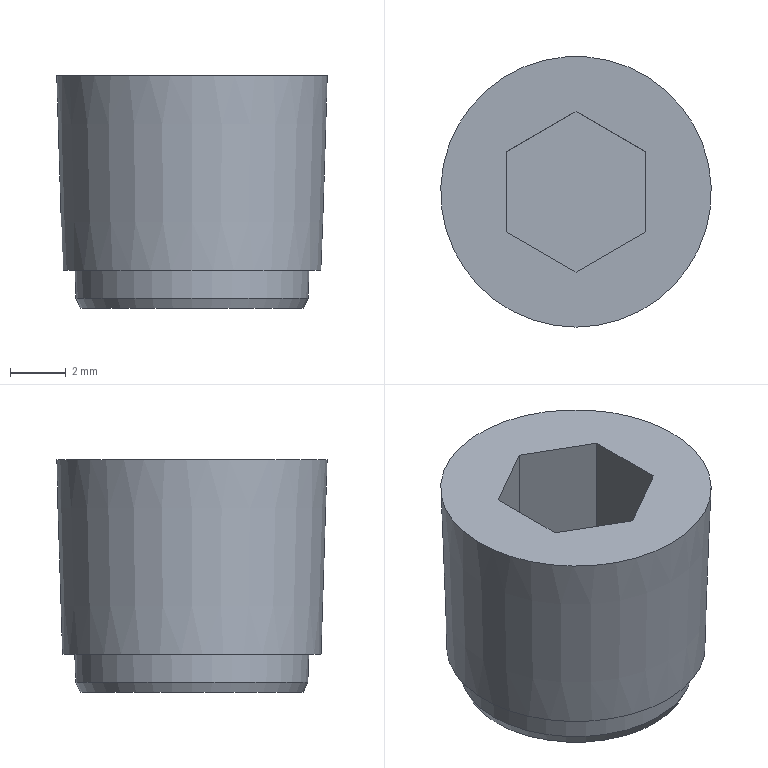Part | STEP file | EM31800001 | 1 solid | 13 faces | box 9.728 x 9.728 x 8.365 mm | volume 484.697 mm3 | plane 10 | cone 3
STEP:
#1=CARTESIAN_POINT('',(0.,0.,0.));
#2=DIRECTION('',(0.,0.,1.));
#3=DIRECTION('',(1.,0.,0.));
#4=AXIS2_PLACEMENT_3D('',#1,#2,#3);
#5=CARTESIAN_POINT('',(0.,-4.864,0.));
#6=VERTEX_POINT('',#5);
#7=CARTESIAN_POINT('',(0.,0.,0.));
#8=DIRECTION('',(0.,0.,-1.));
#9=DIRECTION('',(0.,-1.,0.));
#10=AXIS2_PLACEMENT_3D('',#7,#8,#9);
#11=CIRCLE('',#10,4.864);
#12=CARTESIAN_POINT('',(0.,0.,0.));
#13=DIRECTION('',(0.,0.,-1.));
#14=DIRECTION('',(0.,-1.,0.));
#15=AXIS2_PLACEMENT_3D('',#12,#13,#14);
#16=PLANE('',#15);
#17=CARTESIAN_POINT('',(0.,0.));
#18=DIRECTION('',(1.,0.));
#19=AXIS2_PLACEMENT_2D('',#17,#18);
#20=CIRCLE('',#19,4.864);
#21=(GEOMETRIC_REPRESENTATION_CONTEXT(2)PARAMETRIC_REPRESENTATION_CONTEXT()REPRESENTATION_CONTEXT('',''));
#22=DEFINITIONAL_REPRESENTATION('',(#20),#21);
#23=PCURVE('',#16,#22);
#24=CARTESIAN_POINT('',(0.,0.,-6.997));
#25=DIRECTION('',(0.,0.,1.));
#26=DIRECTION('',(0.,1.,0.));
#27=AXIS2_PLACEMENT_3D('',#24,#25,#26);
#28=CONICAL_SURFACE('',#27,4.644,0.03142);
#29=CARTESIAN_POINT('',(9.425,6.997));
#30=DIRECTION('',(-1.,0.));
#31=VECTOR('',#30,1.);
#32=LINE('',#29,#31);
#33=(GEOMETRIC_REPRESENTATION_CONTEXT(2)PARAMETRIC_REPRESENTATION_CONTEXT()REPRESENTATION_CONTEXT('',''));
#34=DEFINITIONAL_REPRESENTATION('',(#32),#33);
#35=PCURVE('',#28,#34);
#36=SURFACE_CURVE('',#11,(#23,#35),.PCURVE_S1.);
#37=EDGE_CURVE('',#6,#6,#36,.T.);
#38=ORIENTED_EDGE('',*,*,#37,.F.);
#39=EDGE_LOOP('',(#38));
#40=FACE_BOUND('',#39,.T.);
#41=CARTESIAN_POINT('',(0.,2.887,0.));
#42=VERTEX_POINT('',#41);
#43=CARTESIAN_POINT('',(-2.5,1.443,0.));
#44=VERTEX_POINT('',#43);
#45=CARTESIAN_POINT('',(-1.25,2.165,0.));
#46=DIRECTION('',(-0.866,-0.5,0.));
#47=VECTOR('',#46,1.);
#48=LINE('',#45,#47);
#49=CARTESIAN_POINT('',(-2.165,1.25));
#50=DIRECTION('',(0.5,0.866));
#51=VECTOR('',#50,1.);
#52=LINE('',#49,#51);
#53=(GEOMETRIC_REPRESENTATION_CONTEXT(2)PARAMETRIC_REPRESENTATION_CONTEXT()REPRESENTATION_CONTEXT('',''));
#54=DEFINITIONAL_REPRESENTATION('',(#52),#53);
#55=PCURVE('',#16,#54);
#56=CARTESIAN_POINT('',(-2.5,1.443,-5.));
#57=DIRECTION('',(0.5,-0.866,0.));
#58=DIRECTION('',(-0.866,-0.5,0.));
#59=AXIS2_PLACEMENT_3D('',#56,#57,#58);
#60=PLANE('',#59);
#61=CARTESIAN_POINT('',(-1.443,-5.));
#62=DIRECTION('',(1.,0.));
#63=VECTOR('',#62,1.);
#64=LINE('',#61,#63);
#65=(GEOMETRIC_REPRESENTATION_CONTEXT(2)PARAMETRIC_REPRESENTATION_CONTEXT()REPRESENTATION_CONTEXT('',''));
#66=DEFINITIONAL_REPRESENTATION('',(#64),#65);
#67=PCURVE('',#60,#66);
#68=SURFACE_CURVE('',#48,(#55,#67),.PCURVE_S1.);
#69=EDGE_CURVE('',#42,#44,#68,.T.);
#70=ORIENTED_EDGE('',*,*,#69,.F.);
#71=CARTESIAN_POINT('',(2.5,1.443,0.));
#72=VERTEX_POINT('',#71);
#73=CARTESIAN_POINT('',(1.25,2.165,0.));
#74=DIRECTION('',(-0.866,0.5,0.));
#75=VECTOR('',#74,1.);
#76=LINE('',#73,#75);
#77=CARTESIAN_POINT('',(-2.165,-1.25));
#78=DIRECTION('',(-0.5,0.866));
#79=VECTOR('',#78,1.);
#80=LINE('',#77,#79);
#81=(GEOMETRIC_REPRESENTATION_CONTEXT(2)PARAMETRIC_REPRESENTATION_CONTEXT()REPRESENTATION_CONTEXT('',''));
#82=DEFINITIONAL_REPRESENTATION('',(#80),#81);
#83=PCURVE('',#16,#82);
#84=CARTESIAN_POINT('',(0.,2.887,-5.));
#85=DIRECTION('',(-0.5,-0.866,0.));
#86=DIRECTION('',(-0.866,0.5,0.));
#87=AXIS2_PLACEMENT_3D('',#84,#85,#86);
#88=PLANE('',#87);
#89=CARTESIAN_POINT('',(-1.443,-5.));
#90=DIRECTION('',(1.,0.));
#91=VECTOR('',#90,1.);
#92=LINE('',#89,#91);
#93=(GEOMETRIC_REPRESENTATION_CONTEXT(2)PARAMETRIC_REPRESENTATION_CONTEXT()REPRESENTATION_CONTEXT('',''));
#94=DEFINITIONAL_REPRESENTATION('',(#92),#93);
#95=PCURVE('',#88,#94);
#96=SURFACE_CURVE('',#76,(#83,#95),.PCURVE_S1.);
#97=EDGE_CURVE('',#72,#42,#96,.T.);
#98=ORIENTED_EDGE('',*,*,#97,.F.);
#99=CARTESIAN_POINT('',(2.5,-1.443,0.));
#100=VERTEX_POINT('',#99);
#101=CARTESIAN_POINT('',(2.5,0.,0.));
#102=DIRECTION('',(0.,1.,0.));
#103=VECTOR('',#102,1.);
#104=LINE('',#101,#103);
#105=CARTESIAN_POINT('',(0.,-2.5));
#106=DIRECTION('',(-1.,0.));
#107=VECTOR('',#106,1.);
#108=LINE('',#105,#107);
#109=(GEOMETRIC_REPRESENTATION_CONTEXT(2)PARAMETRIC_REPRESENTATION_CONTEXT()REPRESENTATION_CONTEXT('',''));
#110=DEFINITIONAL_REPRESENTATION('',(#108),#109);
#111=PCURVE('',#16,#110);
#112=CARTESIAN_POINT('',(2.5,1.443,-5.));
#113=DIRECTION('',(-1.,0.,0.));
#114=DIRECTION('',(0.,1.,0.));
#115=AXIS2_PLACEMENT_3D('',#112,#113,#114);
#116=PLANE('',#115);
#117=CARTESIAN_POINT('',(-1.443,-5.));
#118=DIRECTION('',(1.,0.));
#119=VECTOR('',#118,1.);
#120=LINE('',#117,#119);
#121=(GEOMETRIC_REPRESENTATION_CONTEXT(2)PARAMETRIC_REPRESENTATION_CONTEXT()REPRESENTATION_CONTEXT('',''));
#122=DEFINITIONAL_REPRESENTATION('',(#120),#121);
#123=PCURVE('',#116,#122);
#124=SURFACE_CURVE('',#104,(#111,#123),.PCURVE_S1.);
#125=EDGE_CURVE('',#100,#72,#124,.T.);
#126=ORIENTED_EDGE('',*,*,#125,.F.);
#127=CARTESIAN_POINT('',(0.,-2.887,0.));
#128=VERTEX_POINT('',#127);
#129=CARTESIAN_POINT('',(1.25,-2.165,0.));
#130=DIRECTION('',(0.866,0.5,0.));
#131=VECTOR('',#130,1.);
#132=LINE('',#129,#131);
#133=CARTESIAN_POINT('',(2.165,-1.25));
#134=DIRECTION('',(-0.5,-0.866));
#135=VECTOR('',#134,1.);
#136=LINE('',#133,#135);
#137=(GEOMETRIC_REPRESENTATION_CONTEXT(2)PARAMETRIC_REPRESENTATION_CONTEXT()REPRESENTATION_CONTEXT('',''));
#138=DEFINITIONAL_REPRESENTATION('',(#136),#137);
#139=PCURVE('',#16,#138);
#140=CARTESIAN_POINT('',(2.5,-1.443,-5.));
#141=DIRECTION('',(-0.5,0.866,0.));
#142=DIRECTION('',(0.866,0.5,0.));
#143=AXIS2_PLACEMENT_3D('',#140,#141,#142);
#144=PLANE('',#143);
#145=CARTESIAN_POINT('',(-1.443,-5.));
#146=DIRECTION('',(1.,0.));
#147=VECTOR('',#146,1.);
#148=LINE('',#145,#147);
#149=(GEOMETRIC_REPRESENTATION_CONTEXT(2)PARAMETRIC_REPRESENTATION_CONTEXT()REPRESENTATION_CONTEXT('',''));
#150=DEFINITIONAL_REPRESENTATION('',(#148),#149);
#151=PCURVE('',#144,#150);
#152=SURFACE_CURVE('',#132,(#139,#151),.PCURVE_S1.);
#153=EDGE_CURVE('',#128,#100,#152,.T.);
#154=ORIENTED_EDGE('',*,*,#153,.F.);
#155=CARTESIAN_POINT('',(-2.5,-1.443,0.));
#156=VERTEX_POINT('',#155);
#157=CARTESIAN_POINT('',(-1.25,-2.165,0.));
#158=DIRECTION('',(0.866,-0.5,0.));
#159=VECTOR('',#158,1.);
#160=LINE('',#157,#159);
#161=CARTESIAN_POINT('',(2.165,1.25));
#162=DIRECTION('',(0.5,-0.866));
#163=VECTOR('',#162,1.);
#164=LINE('',#161,#163);
#165=(GEOMETRIC_REPRESENTATION_CONTEXT(2)PARAMETRIC_REPRESENTATION_CONTEXT()REPRESENTATION_CONTEXT('',''));
#166=DEFINITIONAL_REPRESENTATION('',(#164),#165);
#167=PCURVE('',#16,#166);
#168=CARTESIAN_POINT('',(0.,-2.887,-5.));
#169=DIRECTION('',(0.5,0.866,0.));
#170=DIRECTION('',(0.866,-0.5,0.));
#171=AXIS2_PLACEMENT_3D('',#168,#169,#170);
#172=PLANE('',#171);
#173=CARTESIAN_POINT('',(-1.443,-5.));
#174=DIRECTION('',(1.,0.));
#175=VECTOR('',#174,1.);
#176=LINE('',#173,#175);
#177=(GEOMETRIC_REPRESENTATION_CONTEXT(2)PARAMETRIC_REPRESENTATION_CONTEXT()REPRESENTATION_CONTEXT('',''));
#178=DEFINITIONAL_REPRESENTATION('',(#176),#177);
#179=PCURVE('',#172,#178);
#180=SURFACE_CURVE('',#160,(#167,#179),.PCURVE_S1.);
#181=EDGE_CURVE('',#156,#128,#180,.T.);
#182=ORIENTED_EDGE('',*,*,#181,.F.);
#183=CARTESIAN_POINT('',(-2.5,0.,0.));
#184=DIRECTION('',(0.,-1.,0.));
#185=VECTOR('',#184,1.);
#186=LINE('',#183,#185);
#187=CARTESIAN_POINT('',(0.,2.5));
#188=DIRECTION('',(1.,0.));
#189=VECTOR('',#188,1.);
#190=LINE('',#187,#189);
#191=(GEOMETRIC_REPRESENTATION_CONTEXT(2)PARAMETRIC_REPRESENTATION_CONTEXT()REPRESENTATION_CONTEXT('',''));
#192=DEFINITIONAL_REPRESENTATION('',(#190),#191);
#193=PCURVE('',#16,#192);
#194=CARTESIAN_POINT('',(-2.5,-1.443,-5.));
#195=DIRECTION('',(1.,0.,0.));
#196=DIRECTION('',(0.,-1.,0.));
#197=AXIS2_PLACEMENT_3D('',#194,#195,#196);
#198=PLANE('',#197);
#199=CARTESIAN_POINT('',(-1.443,-5.));
#200=DIRECTION('',(1.,0.));
#201=VECTOR('',#200,1.);
#202=LINE('',#199,#201);
#203=(GEOMETRIC_REPRESENTATION_CONTEXT(2)PARAMETRIC_REPRESENTATION_CONTEXT()REPRESENTATION_CONTEXT('',''));
#204=DEFINITIONAL_REPRESENTATION('',(#202),#203);
#205=PCURVE('',#198,#204);
#206=SURFACE_CURVE('',#186,(#193,#205),.PCURVE_S1.);
#207=EDGE_CURVE('',#44,#156,#206,.T.);
#208=ORIENTED_EDGE('',*,*,#207,.F.);
#209=EDGE_LOOP('',(#70,#98,#126,#154,#182,#208));
#210=FACE_BOUND('',#209,.T.);
#211=ADVANCED_FACE('',(#40,#210),#16,.F.);
#212=CARTESIAN_POINT('',(0.,-4.644,-6.997));
#213=VERTEX_POINT('',#212);
#214=CARTESIAN_POINT('',(0.,0.,-6.997));
#215=DIRECTION('',(0.,0.,-1.));
#216=DIRECTION('',(0.,-1.,0.));
#217=AXIS2_PLACEMENT_3D('',#214,#215,#216);
#218=CIRCLE('',#217,4.644);
#219=CARTESIAN_POINT('',(0.,0.,-6.997));
#220=DIRECTION('',(0.,0.,-1.));
#221=DIRECTION('',(0.,-1.,0.));
#222=AXIS2_PLACEMENT_3D('',#219,#220,#221);
#223=PLANE('',#222);
#224=CARTESIAN_POINT('',(0.,0.));
#225=DIRECTION('',(1.,0.));
#226=AXIS2_PLACEMENT_2D('',#224,#225);
#227=CIRCLE('',#226,4.644);
#228=(GEOMETRIC_REPRESENTATION_CONTEXT(2)PARAMETRIC_REPRESENTATION_CONTEXT()REPRESENTATION_CONTEXT('',''));
#229=DEFINITIONAL_REPRESENTATION('',(#227),#228);
#230=PCURVE('',#223,#229);
#231=CARTESIAN_POINT('',(9.425,0.));
#232=DIRECTION('',(-1.,0.));
#233=VECTOR('',#232,1.);
#234=LINE('',#231,#233);
#235=(GEOMETRIC_REPRESENTATION_CONTEXT(2)PARAMETRIC_REPRESENTATION_CONTEXT()REPRESENTATION_CONTEXT('',''));
#236=DEFINITIONAL_REPRESENTATION('',(#234),#235);
#237=PCURVE('',#28,#236);
#238=SURFACE_CURVE('',#218,(#230,#237),.PCURVE_S1.);
#239=EDGE_CURVE('',#213,#213,#238,.T.);
#240=ORIENTED_EDGE('',*,*,#239,.T.);
#241=EDGE_LOOP('',(#240));
#242=FACE_BOUND('',#241,.T.);
#243=CARTESIAN_POINT('',(0.,-4.204,-6.997));
#244=VERTEX_POINT('',#243);
#245=CARTESIAN_POINT('',(0.,0.,-6.997));
#246=DIRECTION('',(0.,0.,1.));
#247=DIRECTION('',(0.,-1.,0.));
#248=AXIS2_PLACEMENT_3D('',#245,#246,#247);
#249=CIRCLE('',#248,4.204);
#250=CARTESIAN_POINT('',(4.204,0.));
#251=CARTESIAN_POINT('',(4.204,-7.281));
#252=CARTESIAN_POINT('',(-2.102,-3.641));
#253=CARTESIAN_POINT('',(-8.407,0.));
#254=CARTESIAN_POINT('',(-2.102,3.641));
#255=CARTESIAN_POINT('',(4.204,7.281));
#256=CARTESIAN_POINT('',(4.204,0.));
#257=(BOUNDED_CURVE()B_SPLINE_CURVE(2,(#250,#251,#252,#253,#254,#255,#256),.UNSPECIFIED.,.T.,.F.)B_SPLINE_CURVE_WITH_KNOTS((1,2,2,2,2,1),(-2.094,0.,2.094,4.189,6.283,8.378),.UNSPECIFIED.)CURVE()GEOMETRIC_REPRESENTATION_ITEM()RATIONAL_B_SPLINE_CURVE((1.,0.5,1.,0.5,1.,0.5,1.))REPRESENTATION_ITEM(''));
#258=(GEOMETRIC_REPRESENTATION_CONTEXT(2)PARAMETRIC_REPRESENTATION_CONTEXT()REPRESENTATION_CONTEXT('',''));
#259=DEFINITIONAL_REPRESENTATION('',(#257),#258);
#260=PCURVE('',#223,#259);
#261=CARTESIAN_POINT('',(0.,0.,-7.997));
#262=DIRECTION('',(0.,0.,1.));
#263=DIRECTION('',(0.,1.,0.));
#264=AXIS2_PLACEMENT_3D('',#261,#262,#263);
#265=CONICAL_SURFACE('',#264,4.172,0.03142);
#266=CARTESIAN_POINT('',(3.142,1.001));
#267=DIRECTION('',(1.,0.));
#268=VECTOR('',#267,1.);
#269=LINE('',#266,#268);
#270=(GEOMETRIC_REPRESENTATION_CONTEXT(2)PARAMETRIC_REPRESENTATION_CONTEXT()REPRESENTATION_CONTEXT('',''));
#271=DEFINITIONAL_REPRESENTATION('',(#269),#270);
#272=PCURVE('',#265,#271);
#273=SURFACE_CURVE('',#249,(#260,#272),.PCURVE_S1.);
#274=EDGE_CURVE('',#244,#244,#273,.T.);
#275=ORIENTED_EDGE('',*,*,#274,.T.);
#276=EDGE_LOOP('',(#275));
#277=FACE_BOUND('',#276,.T.);
#278=ADVANCED_FACE('',(#242,#277),#223,.T.);
#279=ORIENTED_EDGE('',*,*,#37,.T.);
#280=CARTESIAN_POINT('',(0.,-4.644,-6.997));
#281=CARTESIAN_POINT('',(0.,-4.864,0.));
#282=B_SPLINE_CURVE_WITH_KNOTS('',1,(#280,#281),.UNSPECIFIED.,.F.,.F.,(2,2),(0.,7.),.PIECEWISE_BEZIER_KNOTS.);
#283=CARTESIAN_POINT('',(3.142,0.));
#284=DIRECTION('',(0.,1.));
#285=VECTOR('',#284,1.);
#286=LINE('',#283,#285);
#287=(GEOMETRIC_REPRESENTATION_CONTEXT(2)PARAMETRIC_REPRESENTATION_CONTEXT()REPRESENTATION_CONTEXT('',''));
#288=DEFINITIONAL_REPRESENTATION('',(#286),#287);
#289=PCURVE('',#28,#288);
#290=CARTESIAN_POINT('',(9.425,0.));
#291=DIRECTION('',(0.,1.));
#292=VECTOR('',#291,1.);
#293=LINE('',#290,#292);
#294=(GEOMETRIC_REPRESENTATION_CONTEXT(2)PARAMETRIC_REPRESENTATION_CONTEXT()REPRESENTATION_CONTEXT('',''));
#295=DEFINITIONAL_REPRESENTATION('',(#293),#294);
#296=PCURVE('',#28,#295);
#297=SEAM_CURVE('',#282,(#289,#296),.PCURVE_S1.);
#298=EDGE_CURVE('',#213,#6,#297,.T.);
#299=ORIENTED_EDGE('',*,*,#298,.F.);
#300=ORIENTED_EDGE('',*,*,#239,.F.);
#301=ORIENTED_EDGE('',*,*,#298,.T.);
#302=EDGE_LOOP('',(#279,#299,#300,#301));
#303=FACE_BOUND('',#302,.T.);
#304=ADVANCED_FACE('',(#303),#28,.T.);
#305=ORIENTED_EDGE('',*,*,#274,.F.);
#306=CARTESIAN_POINT('',(0.,-4.172,-7.997));
#307=VERTEX_POINT('',#306);
#308=CARTESIAN_POINT('',(0.,-4.172,-7.997));
#309=CARTESIAN_POINT('',(0.,-4.204,-6.997));
#310=B_SPLINE_CURVE_WITH_KNOTS('',1,(#308,#309),.UNSPECIFIED.,.F.,.F.,(2,2),(0.,1.001),.PIECEWISE_BEZIER_KNOTS.);
#311=CARTESIAN_POINT('',(3.142,0.));
#312=DIRECTION('',(0.,1.));
#313=VECTOR('',#312,1.);
#314=LINE('',#311,#313);
#315=(GEOMETRIC_REPRESENTATION_CONTEXT(2)PARAMETRIC_REPRESENTATION_CONTEXT()REPRESENTATION_CONTEXT('',''));
#316=DEFINITIONAL_REPRESENTATION('',(#314),#315);
#317=PCURVE('',#265,#316);
#318=CARTESIAN_POINT('',(9.425,0.));
#319=DIRECTION('',(0.,1.));
#320=VECTOR('',#319,1.);
#321=LINE('',#318,#320);
#322=(GEOMETRIC_REPRESENTATION_CONTEXT(2)PARAMETRIC_REPRESENTATION_CONTEXT()REPRESENTATION_CONTEXT('',''));
#323=DEFINITIONAL_REPRESENTATION('',(#321),#322);
#324=PCURVE('',#265,#323);
#325=SEAM_CURVE('',#310,(#317,#324),.PCURVE_S1.);
#326=EDGE_CURVE('',#307,#244,#325,.T.);
#327=ORIENTED_EDGE('',*,*,#326,.F.);
#328=CARTESIAN_POINT('',(0.,0.,-7.997));
#329=DIRECTION('',(0.,0.,-1.));
#330=DIRECTION('',(0.,-1.,0.));
#331=AXIS2_PLACEMENT_3D('',#328,#329,#330);
#332=CIRCLE('',#331,4.172);
#333=CARTESIAN_POINT('',(9.425,0.));
#334=DIRECTION('',(-1.,0.));
#335=VECTOR('',#334,1.);
#336=LINE('',#333,#335);
#337=(GEOMETRIC_REPRESENTATION_CONTEXT(2)PARAMETRIC_REPRESENTATION_CONTEXT()REPRESENTATION_CONTEXT('',''));
#338=DEFINITIONAL_REPRESENTATION('',(#336),#337);
#339=PCURVE('',#265,#338);
#340=CARTESIAN_POINT('',(0.,0.,-8.365));
#341=DIRECTION('',(0.,0.,1.));
#342=DIRECTION('',(0.,1.,0.));
#343=AXIS2_PLACEMENT_3D('',#340,#341,#342);
#344=CONICAL_SURFACE('',#343,4.,0.4379);
#345=CARTESIAN_POINT('',(9.425,0.3679));
#346=DIRECTION('',(-1.,0.));
#347=VECTOR('',#346,1.);
#348=LINE('',#345,#347);
#349=(GEOMETRIC_REPRESENTATION_CONTEXT(2)PARAMETRIC_REPRESENTATION_CONTEXT()REPRESENTATION_CONTEXT('',''));
#350=DEFINITIONAL_REPRESENTATION('',(#348),#349);
#351=PCURVE('',#344,#350);
#352=SURFACE_CURVE('',#332,(#339,#351),.PCURVE_S1.);
#353=EDGE_CURVE('',#307,#307,#352,.T.);
#354=ORIENTED_EDGE('',*,*,#353,.F.);
#355=ORIENTED_EDGE('',*,*,#326,.T.);
#356=EDGE_LOOP('',(#305,#327,#354,#355));
#357=FACE_BOUND('',#356,.T.);
#358=ADVANCED_FACE('',(#357),#265,.T.);
#359=ORIENTED_EDGE('',*,*,#353,.T.);
#360=CARTESIAN_POINT('',(0.,-4.,-8.365));
#361=VERTEX_POINT('',#360);
#362=CARTESIAN_POINT('',(0.,-4.,-8.365));
#363=CARTESIAN_POINT('',(0.,-4.172,-7.997));
#364=B_SPLINE_CURVE_WITH_KNOTS('',1,(#362,#363),.UNSPECIFIED.,.F.,.F.,(2,2),(0.,0.4063),.PIECEWISE_BEZIER_KNOTS.);
#365=CARTESIAN_POINT('',(3.142,0.));
#366=DIRECTION('',(0.,1.));
#367=VECTOR('',#366,1.);
#368=LINE('',#365,#367);
#369=(GEOMETRIC_REPRESENTATION_CONTEXT(2)PARAMETRIC_REPRESENTATION_CONTEXT()REPRESENTATION_CONTEXT('',''));
#370=DEFINITIONAL_REPRESENTATION('',(#368),#369);
#371=PCURVE('',#344,#370);
#372=CARTESIAN_POINT('',(9.425,0.));
#373=DIRECTION('',(0.,1.));
#374=VECTOR('',#373,1.);
#375=LINE('',#372,#374);
#376=(GEOMETRIC_REPRESENTATION_CONTEXT(2)PARAMETRIC_REPRESENTATION_CONTEXT()REPRESENTATION_CONTEXT('',''));
#377=DEFINITIONAL_REPRESENTATION('',(#375),#376);
#378=PCURVE('',#344,#377);
#379=SEAM_CURVE('',#364,(#371,#378),.PCURVE_S1.);
#380=EDGE_CURVE('',#361,#307,#379,.T.);
#381=ORIENTED_EDGE('',*,*,#380,.F.);
#382=CARTESIAN_POINT('',(0.,0.,-8.365));
#383=DIRECTION('',(0.,0.,-1.));
#384=DIRECTION('',(0.,-1.,0.));
#385=AXIS2_PLACEMENT_3D('',#382,#383,#384);
#386=CIRCLE('',#385,4.);
#387=CARTESIAN_POINT('',(9.425,0.));
#388=DIRECTION('',(-1.,0.));
#389=VECTOR('',#388,1.);
#390=LINE('',#387,#389);
#391=(GEOMETRIC_REPRESENTATION_CONTEXT(2)PARAMETRIC_REPRESENTATION_CONTEXT()REPRESENTATION_CONTEXT('',''));
#392=DEFINITIONAL_REPRESENTATION('',(#390),#391);
#393=PCURVE('',#344,#392);
#394=CARTESIAN_POINT('',(0.,0.,-8.365));
#395=DIRECTION('',(0.,0.,-1.));
#396=DIRECTION('',(0.,-1.,0.));
#397=AXIS2_PLACEMENT_3D('',#394,#395,#396);
#398=PLANE('',#397);
#399=CARTESIAN_POINT('',(0.,0.));
#400=DIRECTION('',(1.,0.));
#401=AXIS2_PLACEMENT_2D('',#399,#400);
#402=CIRCLE('',#401,4.);
#403=(GEOMETRIC_REPRESENTATION_CONTEXT(2)PARAMETRIC_REPRESENTATION_CONTEXT()REPRESENTATION_CONTEXT('',''));
#404=DEFINITIONAL_REPRESENTATION('',(#402),#403);
#405=PCURVE('',#398,#404);
#406=SURFACE_CURVE('',#386,(#393,#405),.PCURVE_S1.);
#407=EDGE_CURVE('',#361,#361,#406,.T.);
#408=ORIENTED_EDGE('',*,*,#407,.F.);
#409=ORIENTED_EDGE('',*,*,#380,.T.);
#410=EDGE_LOOP('',(#359,#381,#408,#409));
#411=FACE_BOUND('',#410,.T.);
#412=ADVANCED_FACE('',(#411),#344,.T.);
#413=ORIENTED_EDGE('',*,*,#407,.T.);
#414=EDGE_LOOP('',(#413));
#415=FACE_BOUND('',#414,.T.);
#416=ADVANCED_FACE('',(#415),#398,.T.);
#417=ORIENTED_EDGE('',*,*,#69,.T.);
#418=CARTESIAN_POINT('',(-2.5,1.443,-4.));
#419=VERTEX_POINT('',#418);
#420=CARTESIAN_POINT('',(-2.5,1.443,-5.));
#421=DIRECTION('',(0.,0.,1.));
#422=VECTOR('',#421,1.);
#423=LINE('',#420,#422);
#424=CARTESIAN_POINT('',(0.,0.));
#425=DIRECTION('',(0.,-1.));
#426=VECTOR('',#425,1.);
#427=LINE('',#424,#426);
#428=(GEOMETRIC_REPRESENTATION_CONTEXT(2)PARAMETRIC_REPRESENTATION_CONTEXT()REPRESENTATION_CONTEXT('',''));
#429=DEFINITIONAL_REPRESENTATION('',(#427),#428);
#430=PCURVE('',#60,#429);
#431=CARTESIAN_POINT('',(-2.887,0.));
#432=DIRECTION('',(0.,-1.));
#433=VECTOR('',#432,1.);
#434=LINE('',#431,#433);
#435=(GEOMETRIC_REPRESENTATION_CONTEXT(2)PARAMETRIC_REPRESENTATION_CONTEXT()REPRESENTATION_CONTEXT('',''));
#436=DEFINITIONAL_REPRESENTATION('',(#434),#435);
#437=PCURVE('',#198,#436);
#438=SURFACE_CURVE('',#423,(#430,#437),.PCURVE_S1.);
#439=EDGE_CURVE('',#419,#44,#438,.T.);
#440=ORIENTED_EDGE('',*,*,#439,.F.);
#441=CARTESIAN_POINT('',(0.,2.887,-4.));
#442=VERTEX_POINT('',#441);
#443=CARTESIAN_POINT('',(-1.25,2.165,-4.));
#444=DIRECTION('',(0.866,0.5,0.));
#445=VECTOR('',#444,1.);
#446=LINE('',#443,#445);
#447=CARTESIAN_POINT('',(-1.443,-1.));
#448=DIRECTION('',(-1.,0.));
#449=VECTOR('',#448,1.);
#450=LINE('',#447,#449);
#451=(GEOMETRIC_REPRESENTATION_CONTEXT(2)PARAMETRIC_REPRESENTATION_CONTEXT()REPRESENTATION_CONTEXT('',''));
#452=DEFINITIONAL_REPRESENTATION('',(#450),#451);
#453=PCURVE('',#60,#452);
#454=CARTESIAN_POINT('',(-1.25,2.165,-4.));
#455=DIRECTION('',(0.,0.,1.));
#456=DIRECTION('',(0.,1.,0.));
#457=AXIS2_PLACEMENT_3D('',#454,#455,#456);
#458=PLANE('',#457);
#459=CARTESIAN_POINT('',(0.,0.));
#460=DIRECTION('',(0.5,-0.866));
#461=VECTOR('',#460,1.);
#462=LINE('',#459,#461);
#463=(GEOMETRIC_REPRESENTATION_CONTEXT(2)PARAMETRIC_REPRESENTATION_CONTEXT()REPRESENTATION_CONTEXT('',''));
#464=DEFINITIONAL_REPRESENTATION('',(#462),#463);
#465=PCURVE('',#458,#464);
#466=SURFACE_CURVE('',#446,(#453,#465),.PCURVE_S1.);
#467=EDGE_CURVE('',#419,#442,#466,.T.);
#468=ORIENTED_EDGE('',*,*,#467,.T.);
#469=CARTESIAN_POINT('',(0.,2.887,-5.));
#470=DIRECTION('',(0.,0.,1.));
#471=VECTOR('',#470,1.);
#472=LINE('',#469,#471);
#473=CARTESIAN_POINT('',(-2.887,0.));
#474=DIRECTION('',(0.,-1.));
#475=VECTOR('',#474,1.);
#476=LINE('',#473,#475);
#477=(GEOMETRIC_REPRESENTATION_CONTEXT(2)PARAMETRIC_REPRESENTATION_CONTEXT()REPRESENTATION_CONTEXT('',''));
#478=DEFINITIONAL_REPRESENTATION('',(#476),#477);
#479=PCURVE('',#60,#478);
#480=CARTESIAN_POINT('',(0.,0.));
#481=DIRECTION('',(0.,-1.));
#482=VECTOR('',#481,1.);
#483=LINE('',#480,#482);
#484=(GEOMETRIC_REPRESENTATION_CONTEXT(2)PARAMETRIC_REPRESENTATION_CONTEXT()REPRESENTATION_CONTEXT('',''));
#485=DEFINITIONAL_REPRESENTATION('',(#483),#484);
#486=PCURVE('',#88,#485);
#487=SURFACE_CURVE('',#472,(#479,#486),.PCURVE_S1.);
#488=EDGE_CURVE('',#442,#42,#487,.T.);
#489=ORIENTED_EDGE('',*,*,#488,.T.);
#490=EDGE_LOOP('',(#417,#440,#468,#489));
#491=FACE_BOUND('',#490,.T.);
#492=ADVANCED_FACE('',(#491),#60,.T.);
#493=ORIENTED_EDGE('',*,*,#97,.T.);
#494=ORIENTED_EDGE('',*,*,#488,.F.);
#495=CARTESIAN_POINT('',(2.5,1.443,-4.));
#496=VERTEX_POINT('',#495);
#497=CARTESIAN_POINT('',(-0.625,3.248,-4.));
#498=DIRECTION('',(0.866,-0.5,0.));
#499=VECTOR('',#498,1.);
#500=LINE('',#497,#499);
#501=CARTESIAN_POINT('',(0.7217,-1.));
#502=DIRECTION('',(-1.,0.));
#503=VECTOR('',#502,1.);
#504=LINE('',#501,#503);
#505=(GEOMETRIC_REPRESENTATION_CONTEXT(2)PARAMETRIC_REPRESENTATION_CONTEXT()REPRESENTATION_CONTEXT('',''));
#506=DEFINITIONAL_REPRESENTATION('',(#504),#505);
#507=PCURVE('',#88,#506);
#508=CARTESIAN_POINT('',(1.083,-0.625));
#509=DIRECTION('',(-0.5,-0.866));
#510=VECTOR('',#509,1.);
#511=LINE('',#508,#510);
#512=(GEOMETRIC_REPRESENTATION_CONTEXT(2)PARAMETRIC_REPRESENTATION_CONTEXT()REPRESENTATION_CONTEXT('',''));
#513=DEFINITIONAL_REPRESENTATION('',(#511),#512);
#514=PCURVE('',#458,#513);
#515=SURFACE_CURVE('',#500,(#507,#514),.PCURVE_S1.);
#516=EDGE_CURVE('',#442,#496,#515,.T.);
#517=ORIENTED_EDGE('',*,*,#516,.T.);
#518=CARTESIAN_POINT('',(2.5,1.443,-5.));
#519=DIRECTION('',(0.,0.,1.));
#520=VECTOR('',#519,1.);
#521=LINE('',#518,#520);
#522=CARTESIAN_POINT('',(-2.887,0.));
#523=DIRECTION('',(0.,-1.));
#524=VECTOR('',#523,1.);
#525=LINE('',#522,#524);
#526=(GEOMETRIC_REPRESENTATION_CONTEXT(2)PARAMETRIC_REPRESENTATION_CONTEXT()REPRESENTATION_CONTEXT('',''));
#527=DEFINITIONAL_REPRESENTATION('',(#525),#526);
#528=PCURVE('',#88,#527);
#529=CARTESIAN_POINT('',(0.,0.));
#530=DIRECTION('',(0.,-1.));
#531=VECTOR('',#530,1.);
#532=LINE('',#529,#531);
#533=(GEOMETRIC_REPRESENTATION_CONTEXT(2)PARAMETRIC_REPRESENTATION_CONTEXT()REPRESENTATION_CONTEXT('',''));
#534=DEFINITIONAL_REPRESENTATION('',(#532),#533);
#535=PCURVE('',#116,#534);
#536=SURFACE_CURVE('',#521,(#528,#535),.PCURVE_S1.);
#537=EDGE_CURVE('',#496,#72,#536,.T.);
#538=ORIENTED_EDGE('',*,*,#537,.T.);
#539=EDGE_LOOP('',(#493,#494,#517,#538));
#540=FACE_BOUND('',#539,.T.);
#541=ADVANCED_FACE('',(#540),#88,.T.);
#542=ORIENTED_EDGE('',*,*,#125,.T.);
#543=ORIENTED_EDGE('',*,*,#537,.F.);
#544=CARTESIAN_POINT('',(2.5,-1.443,-4.));
#545=VERTEX_POINT('',#544);
#546=CARTESIAN_POINT('',(2.5,2.165,-4.));
#547=DIRECTION('',(0.,-1.,0.));
#548=VECTOR('',#547,1.);
#549=LINE('',#546,#548);
#550=CARTESIAN_POINT('',(0.7217,-1.));
#551=DIRECTION('',(-1.,0.));
#552=VECTOR('',#551,1.);
#553=LINE('',#550,#552);
#554=(GEOMETRIC_REPRESENTATION_CONTEXT(2)PARAMETRIC_REPRESENTATION_CONTEXT()REPRESENTATION_CONTEXT('',''));
#555=DEFINITIONAL_REPRESENTATION('',(#553),#554);
#556=PCURVE('',#116,#555);
#557=CARTESIAN_POINT('',(0.,-3.75));
#558=DIRECTION('',(-1.,0.));
#559=VECTOR('',#558,1.);
#560=LINE('',#557,#559);
#561=(GEOMETRIC_REPRESENTATION_CONTEXT(2)PARAMETRIC_REPRESENTATION_CONTEXT()REPRESENTATION_CONTEXT('',''));
#562=DEFINITIONAL_REPRESENTATION('',(#560),#561);
#563=PCURVE('',#458,#562);
#564=SURFACE_CURVE('',#549,(#556,#563),.PCURVE_S1.);
#565=EDGE_CURVE('',#496,#545,#564,.T.);
#566=ORIENTED_EDGE('',*,*,#565,.T.);
#567=CARTESIAN_POINT('',(2.5,-1.443,-5.));
#568=DIRECTION('',(0.,0.,1.));
#569=VECTOR('',#568,1.);
#570=LINE('',#567,#569);
#571=CARTESIAN_POINT('',(-2.887,0.));
#572=DIRECTION('',(0.,-1.));
#573=VECTOR('',#572,1.);
#574=LINE('',#571,#573);
#575=(GEOMETRIC_REPRESENTATION_CONTEXT(2)PARAMETRIC_REPRESENTATION_CONTEXT()REPRESENTATION_CONTEXT('',''));
#576=DEFINITIONAL_REPRESENTATION('',(#574),#575);
#577=PCURVE('',#116,#576);
#578=CARTESIAN_POINT('',(0.,0.));
#579=DIRECTION('',(0.,-1.));
#580=VECTOR('',#579,1.);
#581=LINE('',#578,#580);
#582=(GEOMETRIC_REPRESENTATION_CONTEXT(2)PARAMETRIC_REPRESENTATION_CONTEXT()REPRESENTATION_CONTEXT('',''));
#583=DEFINITIONAL_REPRESENTATION('',(#581),#582);
#584=PCURVE('',#144,#583);
#585=SURFACE_CURVE('',#570,(#577,#584),.PCURVE_S1.);
#586=EDGE_CURVE('',#545,#100,#585,.T.);
#587=ORIENTED_EDGE('',*,*,#586,.T.);
#588=EDGE_LOOP('',(#542,#543,#566,#587));
#589=FACE_BOUND('',#588,.T.);
#590=ADVANCED_FACE('',(#589),#116,.T.);
#591=ORIENTED_EDGE('',*,*,#153,.T.);
#592=ORIENTED_EDGE('',*,*,#586,.F.);
#593=CARTESIAN_POINT('',(0.,-2.887,-4.));
#594=VERTEX_POINT('',#593);
#595=CARTESIAN_POINT('',(1.25,-2.165,-4.));
#596=DIRECTION('',(-0.866,-0.5,0.));
#597=VECTOR('',#596,1.);
#598=LINE('',#595,#597);
#599=CARTESIAN_POINT('',(-1.443,-1.));
#600=DIRECTION('',(-1.,0.));
#601=VECTOR('',#600,1.);
#602=LINE('',#599,#601);
#603=(GEOMETRIC_REPRESENTATION_CONTEXT(2)PARAMETRIC_REPRESENTATION_CONTEXT()REPRESENTATION_CONTEXT('',''));
#604=DEFINITIONAL_REPRESENTATION('',(#602),#603);
#605=PCURVE('',#144,#604);
#606=CARTESIAN_POINT('',(-4.33,-2.5));
#607=DIRECTION('',(-0.5,0.866));
#608=VECTOR('',#607,1.);
#609=LINE('',#606,#608);
#610=(GEOMETRIC_REPRESENTATION_CONTEXT(2)PARAMETRIC_REPRESENTATION_CONTEXT()REPRESENTATION_CONTEXT('',''));
#611=DEFINITIONAL_REPRESENTATION('',(#609),#610);
#612=PCURVE('',#458,#611);
#613=SURFACE_CURVE('',#598,(#605,#612),.PCURVE_S1.);
#614=EDGE_CURVE('',#545,#594,#613,.T.);
#615=ORIENTED_EDGE('',*,*,#614,.T.);
#616=CARTESIAN_POINT('',(0.,-2.887,-5.));
#617=DIRECTION('',(0.,0.,1.));
#618=VECTOR('',#617,1.);
#619=LINE('',#616,#618);
#620=CARTESIAN_POINT('',(-2.887,0.));
#621=DIRECTION('',(0.,-1.));
#622=VECTOR('',#621,1.);
#623=LINE('',#620,#622);
#624=(GEOMETRIC_REPRESENTATION_CONTEXT(2)PARAMETRIC_REPRESENTATION_CONTEXT()REPRESENTATION_CONTEXT('',''));
#625=DEFINITIONAL_REPRESENTATION('',(#623),#624);
#626=PCURVE('',#144,#625);
#627=CARTESIAN_POINT('',(0.,0.));
#628=DIRECTION('',(0.,-1.));
#629=VECTOR('',#628,1.);
#630=LINE('',#627,#629);
#631=(GEOMETRIC_REPRESENTATION_CONTEXT(2)PARAMETRIC_REPRESENTATION_CONTEXT()REPRESENTATION_CONTEXT('',''));
#632=DEFINITIONAL_REPRESENTATION('',(#630),#631);
#633=PCURVE('',#172,#632);
#634=SURFACE_CURVE('',#619,(#626,#633),.PCURVE_S1.);
#635=EDGE_CURVE('',#594,#128,#634,.T.);
#636=ORIENTED_EDGE('',*,*,#635,.T.);
#637=EDGE_LOOP('',(#591,#592,#615,#636));
#638=FACE_BOUND('',#637,.T.);
#639=ADVANCED_FACE('',(#638),#144,.T.);
#640=ORIENTED_EDGE('',*,*,#181,.T.);
#641=ORIENTED_EDGE('',*,*,#635,.F.);
#642=CARTESIAN_POINT('',(-2.5,-1.443,-4.));
#643=VERTEX_POINT('',#642);
#644=CARTESIAN_POINT('',(-3.125,-1.083,-4.));
#645=DIRECTION('',(-0.866,0.5,0.));
#646=VECTOR('',#645,1.);
#647=LINE('',#644,#646);
#648=CARTESIAN_POINT('',(-3.608,-1.));
#649=DIRECTION('',(-1.,0.));
#650=VECTOR('',#649,1.);
#651=LINE('',#648,#650);
#652=(GEOMETRIC_REPRESENTATION_CONTEXT(2)PARAMETRIC_REPRESENTATION_CONTEXT()REPRESENTATION_CONTEXT('',''));
#653=DEFINITIONAL_REPRESENTATION('',(#651),#652);
#654=PCURVE('',#172,#653);
#655=CARTESIAN_POINT('',(-3.248,1.875));
#656=DIRECTION('',(0.5,0.866));
#657=VECTOR('',#656,1.);
#658=LINE('',#655,#657);
#659=(GEOMETRIC_REPRESENTATION_CONTEXT(2)PARAMETRIC_REPRESENTATION_CONTEXT()REPRESENTATION_CONTEXT('',''));
#660=DEFINITIONAL_REPRESENTATION('',(#658),#659);
#661=PCURVE('',#458,#660);
#662=SURFACE_CURVE('',#647,(#654,#661),.PCURVE_S1.);
#663=EDGE_CURVE('',#594,#643,#662,.T.);
#664=ORIENTED_EDGE('',*,*,#663,.T.);
#665=CARTESIAN_POINT('',(-2.5,-1.443,-5.));
#666=DIRECTION('',(0.,0.,1.));
#667=VECTOR('',#666,1.);
#668=LINE('',#665,#667);
#669=CARTESIAN_POINT('',(-2.887,0.));
#670=DIRECTION('',(0.,-1.));
#671=VECTOR('',#670,1.);
#672=LINE('',#669,#671);
#673=(GEOMETRIC_REPRESENTATION_CONTEXT(2)PARAMETRIC_REPRESENTATION_CONTEXT()REPRESENTATION_CONTEXT('',''));
#674=DEFINITIONAL_REPRESENTATION('',(#672),#673);
#675=PCURVE('',#172,#674);
#676=CARTESIAN_POINT('',(0.,0.));
#677=DIRECTION('',(0.,-1.));
#678=VECTOR('',#677,1.);
#679=LINE('',#676,#678);
#680=(GEOMETRIC_REPRESENTATION_CONTEXT(2)PARAMETRIC_REPRESENTATION_CONTEXT()REPRESENTATION_CONTEXT('',''));
#681=DEFINITIONAL_REPRESENTATION('',(#679),#680);
#682=PCURVE('',#198,#681);
#683=SURFACE_CURVE('',#668,(#675,#682),.PCURVE_S1.);
#684=EDGE_CURVE('',#643,#156,#683,.T.);
#685=ORIENTED_EDGE('',*,*,#684,.T.);
#686=EDGE_LOOP('',(#640,#641,#664,#685));
#687=FACE_BOUND('',#686,.T.);
#688=ADVANCED_FACE('',(#687),#172,.T.);
#689=ORIENTED_EDGE('',*,*,#207,.T.);
#690=ORIENTED_EDGE('',*,*,#684,.F.);
#691=CARTESIAN_POINT('',(-2.5,2.165,-4.));
#692=DIRECTION('',(0.,1.,0.));
#693=VECTOR('',#692,1.);
#694=LINE('',#691,#693);
#695=CARTESIAN_POINT('',(-3.608,-1.));
#696=DIRECTION('',(-1.,0.));
#697=VECTOR('',#696,1.);
#698=LINE('',#695,#697);
#699=(GEOMETRIC_REPRESENTATION_CONTEXT(2)PARAMETRIC_REPRESENTATION_CONTEXT()REPRESENTATION_CONTEXT('',''));
#700=DEFINITIONAL_REPRESENTATION('',(#698),#699);
#701=PCURVE('',#198,#700);
#702=CARTESIAN_POINT('',(0.,1.25));
#703=DIRECTION('',(1.,0.));
#704=VECTOR('',#703,1.);
#705=LINE('',#702,#704);
#706=(GEOMETRIC_REPRESENTATION_CONTEXT(2)PARAMETRIC_REPRESENTATION_CONTEXT()REPRESENTATION_CONTEXT('',''));
#707=DEFINITIONAL_REPRESENTATION('',(#705),#706);
#708=PCURVE('',#458,#707);
#709=SURFACE_CURVE('',#694,(#701,#708),.PCURVE_S1.);
#710=EDGE_CURVE('',#643,#419,#709,.T.);
#711=ORIENTED_EDGE('',*,*,#710,.T.);
#712=ORIENTED_EDGE('',*,*,#439,.T.);
#713=EDGE_LOOP('',(#689,#690,#711,#712));
#714=FACE_BOUND('',#713,.T.);
#715=ADVANCED_FACE('',(#714),#198,.T.);
#716=ORIENTED_EDGE('',*,*,#467,.F.);
#717=ORIENTED_EDGE('',*,*,#710,.F.);
#718=ORIENTED_EDGE('',*,*,#663,.F.);
#719=ORIENTED_EDGE('',*,*,#614,.F.);
#720=ORIENTED_EDGE('',*,*,#565,.F.);
#721=ORIENTED_EDGE('',*,*,#516,.F.);
#722=EDGE_LOOP('',(#716,#717,#718,#719,#720,#721));
#723=FACE_BOUND('',#722,.T.);
#724=ADVANCED_FACE('',(#723),#458,.T.);
#725=CLOSED_SHELL('',(#211,#278,#304,#358,#412,#416,#492,#541,#590,#639,#688,#715,#724));
#726=MANIFOLD_SOLID_BREP('',#725);
#727=(LENGTH_UNIT()NAMED_UNIT(*)SI_UNIT(.MILLI.,.METRE.));
#728=UNCERTAINTY_MEASURE_WITH_UNIT(LENGTH_MEASURE(0.000002),#727,'','');
#729=(NAMED_UNIT(*)PLANE_ANGLE_UNIT()SI_UNIT($,.RADIAN.));
#730=(NAMED_UNIT(*)SI_UNIT($,.STERADIAN.)SOLID_ANGLE_UNIT());
#731=(GEOMETRIC_REPRESENTATION_CONTEXT(3)GLOBAL_UNCERTAINTY_ASSIGNED_CONTEXT((#728))GLOBAL_UNIT_ASSIGNED_CONTEXT((#727,#729,#730))REPRESENTATION_CONTEXT('',''));
#732=ADVANCED_BREP_SHAPE_REPRESENTATION('',(#4,#726),#731);